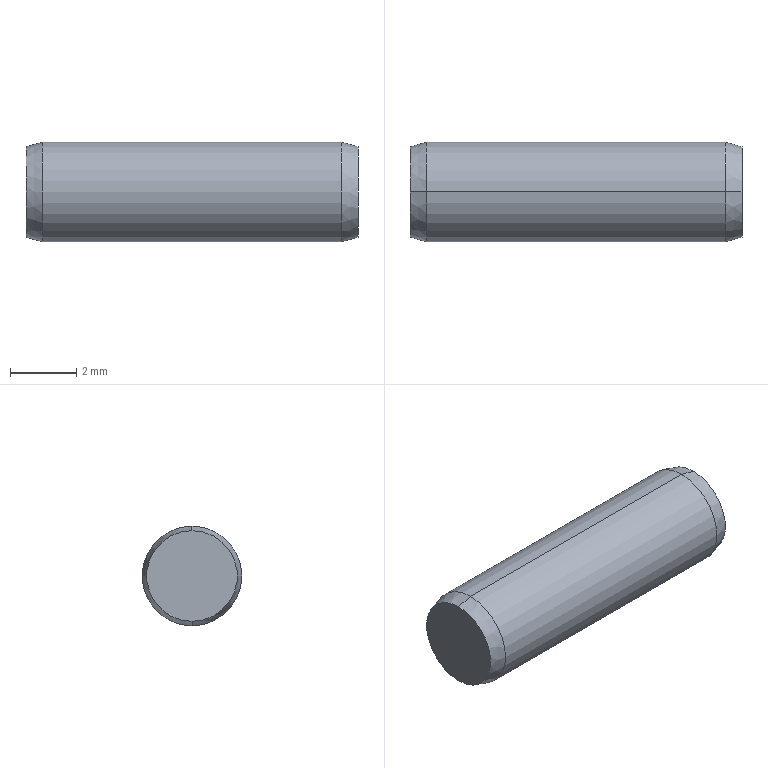Part | NX | features BREP 1 | 1 solid | 8 faces | box 10 x 3 x 3 mm | volume 70.073 mm3 | cone 4 | cylinder 2 | plane 2 | commonest cylinder face diameters 3 x2
STEP:
#1=CARTESIAN_POINT('',(-1.,0.,-1.5));
#2=VERTEX_POINT('',#1);
#3=CARTESIAN_POINT('',(8.,0.,-1.5));
#4=VERTEX_POINT('',#3);
#5=CARTESIAN_POINT('',(0.,0.,-1.5));
#6=DIRECTION('',(-1.,0.,0.));
#7=VECTOR('',#6,1000.);
#8=LINE('',#5,#7);
#9=EDGE_CURVE('',#2,#4,#8,.F.);
#10=ORIENTED_EDGE('',*,*,#9,.T.);
#11=CARTESIAN_POINT('',(8.,0.,1.5));
#12=VERTEX_POINT('',#11);
#13=CARTESIAN_POINT('',(8.,0.,0.));
#14=DIRECTION('',(-1.,0.,0.));
#15=DIRECTION('',(0.,0.,1.));
#16=AXIS2_PLACEMENT_3D('',#13,#14,#15);
#17=CIRCLE('',#16,1.5);
#18=EDGE_CURVE('',#4,#12,#17,.T.);
#19=ORIENTED_EDGE('',*,*,#18,.T.);
#20=CARTESIAN_POINT('',(-1.,0.,1.5));
#21=VERTEX_POINT('',#20);
#22=CARTESIAN_POINT('',(0.,0.,1.5));
#23=DIRECTION('',(-1.,0.,0.));
#24=VECTOR('',#23,1000.);
#25=LINE('',#22,#24);
#26=EDGE_CURVE('',#21,#12,#25,.F.);
#27=ORIENTED_EDGE('',*,*,#26,.F.);
#28=CARTESIAN_POINT('',(-1.,0.,0.));
#29=DIRECTION('',(-1.,0.,0.));
#30=DIRECTION('',(0.,0.,1.));
#31=AXIS2_PLACEMENT_3D('',#28,#29,#30);
#32=CIRCLE('',#31,1.5);
#33=EDGE_CURVE('',#2,#21,#32,.T.);
#34=ORIENTED_EDGE('',*,*,#33,.F.);
#35=EDGE_LOOP('',(#10,#19,#27,#34));
#36=FACE_BOUND('',#35,.T.);
#37=CARTESIAN_POINT('',(0.,0.,0.));
#38=DIRECTION('',(-1.,0.,0.));
#39=DIRECTION('',(0.,0.,1.));
#40=AXIS2_PLACEMENT_3D('',#37,#38,#39);
#41=CYLINDRICAL_SURFACE('',#40,1.5);
#42=ADVANCED_FACE('',(#36),#41,.T.);
#43=CARTESIAN_POINT('',(-1.5,0.,1.366));
#44=VERTEX_POINT('',#43);
#45=CARTESIAN_POINT('',(-1.,0.,1.5));
#46=DIRECTION('',(0.9659,0.,0.2588));
#47=VECTOR('',#46,1000.);
#48=LINE('',#45,#47);
#49=EDGE_CURVE('',#44,#21,#48,.T.);
#50=ORIENTED_EDGE('',*,*,#49,.F.);
#51=CARTESIAN_POINT('',(-1.5,0.,-1.366));
#52=VERTEX_POINT('',#51);
#53=CARTESIAN_POINT('',(-1.5,0.,0.));
#54=DIRECTION('',(-1.,0.,0.));
#55=DIRECTION('',(0.,0.,1.));
#56=AXIS2_PLACEMENT_3D('',#53,#54,#55);
#57=CIRCLE('',#56,1.366);
#58=EDGE_CURVE('',#52,#44,#57,.T.);
#59=ORIENTED_EDGE('',*,*,#58,.F.);
#60=CARTESIAN_POINT('',(-1.,0.,-1.5));
#61=DIRECTION('',(0.9659,0.,-0.2588));
#62=VECTOR('',#61,1000.);
#63=LINE('',#60,#62);
#64=EDGE_CURVE('',#52,#2,#63,.T.);
#65=ORIENTED_EDGE('',*,*,#64,.T.);
#66=ORIENTED_EDGE('',*,*,#33,.T.);
#67=EDGE_LOOP('',(#50,#59,#65,#66));
#68=FACE_BOUND('',#67,.T.);
#69=CARTESIAN_POINT('',(-1.,0.,0.));
#70=DIRECTION('',(1.,0.,0.));
#71=DIRECTION('',(0.,0.,-1.));
#72=AXIS2_PLACEMENT_3D('',#69,#70,#71);
#73=CONICAL_SURFACE('',#72,1.5,0.2618);
#74=ADVANCED_FACE('',(#68),#73,.T.);
#75=ORIENTED_EDGE('',*,*,#58,.T.);
#76=CARTESIAN_POINT('',(-1.5,0.,0.));
#77=DIRECTION('',(-1.,0.,0.));
#78=DIRECTION('',(0.,0.,1.));
#79=AXIS2_PLACEMENT_3D('',#76,#77,#78);
#80=CIRCLE('',#79,1.366);
#81=EDGE_CURVE('',#44,#52,#80,.T.);
#82=ORIENTED_EDGE('',*,*,#81,.T.);
#83=EDGE_LOOP('',(#75,#82));
#84=FACE_BOUND('',#83,.T.);
#85=CARTESIAN_POINT('',(-1.5,1.366,0.));
#86=DIRECTION('',(1.,0.,0.));
#87=DIRECTION('',(0.,0.,-1.));
#88=AXIS2_PLACEMENT_3D('',#85,#86,#87);
#89=PLANE('',#88);
#90=ADVANCED_FACE('',(#84),#89,.F.);
#91=CARTESIAN_POINT('',(8.5,0.,1.366));
#92=VERTEX_POINT('',#91);
#93=CARTESIAN_POINT('',(8.5,0.,-1.366));
#94=VERTEX_POINT('',#93);
#95=CARTESIAN_POINT('',(8.5,0.,0.));
#96=DIRECTION('',(-1.,0.,0.));
#97=DIRECTION('',(0.,0.,1.));
#98=AXIS2_PLACEMENT_3D('',#95,#96,#97);
#99=CIRCLE('',#98,1.366);
#100=EDGE_CURVE('',#92,#94,#99,.T.);
#101=ORIENTED_EDGE('',*,*,#100,.F.);
#102=CARTESIAN_POINT('',(8.5,0.,0.));
#103=DIRECTION('',(-1.,0.,0.));
#104=DIRECTION('',(0.,0.,1.));
#105=AXIS2_PLACEMENT_3D('',#102,#103,#104);
#106=CIRCLE('',#105,1.366);
#107=EDGE_CURVE('',#94,#92,#106,.T.);
#108=ORIENTED_EDGE('',*,*,#107,.F.);
#109=EDGE_LOOP('',(#101,#108));
#110=FACE_BOUND('',#109,.T.);
#111=CARTESIAN_POINT('',(8.5,1.366,0.));
#112=DIRECTION('',(-1.,0.,0.));
#113=DIRECTION('',(0.,0.,1.));
#114=AXIS2_PLACEMENT_3D('',#111,#112,#113);
#115=PLANE('',#114);
#116=ADVANCED_FACE('',(#110),#115,.F.);
#117=CARTESIAN_POINT('',(8.5,0.,-1.366));
#118=DIRECTION('',(-0.9659,0.,-0.2588));
#119=VECTOR('',#118,1000.);
#120=LINE('',#117,#119);
#121=EDGE_CURVE('',#4,#94,#120,.F.);
#122=ORIENTED_EDGE('',*,*,#121,.T.);
#123=ORIENTED_EDGE('',*,*,#107,.T.);
#124=CARTESIAN_POINT('',(8.5,0.,1.366));
#125=DIRECTION('',(-0.9659,0.,0.2588));
#126=VECTOR('',#125,1000.);
#127=LINE('',#124,#126);
#128=EDGE_CURVE('',#12,#92,#127,.F.);
#129=ORIENTED_EDGE('',*,*,#128,.F.);
#130=ORIENTED_EDGE('',*,*,#18,.F.);
#131=EDGE_LOOP('',(#122,#123,#129,#130));
#132=FACE_BOUND('',#131,.T.);
#133=CARTESIAN_POINT('',(8.5,0.,0.));
#134=DIRECTION('',(-1.,0.,0.));
#135=DIRECTION('',(0.,0.,1.));
#136=AXIS2_PLACEMENT_3D('',#133,#134,#135);
#137=CONICAL_SURFACE('',#136,1.366,0.2618);
#138=ADVANCED_FACE('',(#132),#137,.T.);
#139=ORIENTED_EDGE('',*,*,#100,.T.);
#140=ORIENTED_EDGE('',*,*,#121,.F.);
#141=CARTESIAN_POINT('',(8.,0.,0.));
#142=DIRECTION('',(-1.,0.,0.));
#143=DIRECTION('',(0.,0.,1.));
#144=AXIS2_PLACEMENT_3D('',#141,#142,#143);
#145=CIRCLE('',#144,1.5);
#146=EDGE_CURVE('',#12,#4,#145,.T.);
#147=ORIENTED_EDGE('',*,*,#146,.F.);
#148=ORIENTED_EDGE('',*,*,#128,.T.);
#149=EDGE_LOOP('',(#139,#140,#147,#148));
#150=FACE_BOUND('',#149,.T.);
#151=CARTESIAN_POINT('',(8.5,0.,0.));
#152=DIRECTION('',(-1.,0.,0.));
#153=DIRECTION('',(0.,0.,1.));
#154=AXIS2_PLACEMENT_3D('',#151,#152,#153);
#155=CONICAL_SURFACE('',#154,1.366,0.2618);
#156=ADVANCED_FACE('',(#150),#155,.T.);
#157=ORIENTED_EDGE('',*,*,#81,.F.);
#158=ORIENTED_EDGE('',*,*,#49,.T.);
#159=CARTESIAN_POINT('',(-1.,0.,0.));
#160=DIRECTION('',(-1.,0.,0.));
#161=DIRECTION('',(0.,0.,1.));
#162=AXIS2_PLACEMENT_3D('',#159,#160,#161);
#163=CIRCLE('',#162,1.5);
#164=EDGE_CURVE('',#21,#2,#163,.T.);
#165=ORIENTED_EDGE('',*,*,#164,.T.);
#166=ORIENTED_EDGE('',*,*,#64,.F.);
#167=EDGE_LOOP('',(#157,#158,#165,#166));
#168=FACE_BOUND('',#167,.T.);
#169=CARTESIAN_POINT('',(-1.,0.,0.));
#170=DIRECTION('',(1.,0.,0.));
#171=DIRECTION('',(0.,0.,-1.));
#172=AXIS2_PLACEMENT_3D('',#169,#170,#171);
#173=CONICAL_SURFACE('',#172,1.5,0.2618);
#174=ADVANCED_FACE('',(#168),#173,.T.);
#175=ORIENTED_EDGE('',*,*,#146,.T.);
#176=ORIENTED_EDGE('',*,*,#9,.F.);
#177=ORIENTED_EDGE('',*,*,#164,.F.);
#178=ORIENTED_EDGE('',*,*,#26,.T.);
#179=EDGE_LOOP('',(#175,#176,#177,#178));
#180=FACE_BOUND('',#179,.T.);
#181=CARTESIAN_POINT('',(0.,0.,0.));
#182=DIRECTION('',(-1.,0.,0.));
#183=DIRECTION('',(0.,0.,1.));
#184=AXIS2_PLACEMENT_3D('',#181,#182,#183);
#185=CYLINDRICAL_SURFACE('',#184,1.5);
#186=ADVANCED_FACE('',(#180),#185,.T.);
#187=CLOSED_SHELL('',(#42,#74,#90,#116,#138,#156,#174,#186));
#188=MANIFOLD_SOLID_BREP('',#187);
#189=(LENGTH_UNIT()NAMED_UNIT(*)SI_UNIT(.MILLI.,.METRE.));
#190=UNCERTAINTY_MEASURE_WITH_UNIT(LENGTH_MEASURE(0.00001),#189,'','');
#191=(NAMED_UNIT(*)PLANE_ANGLE_UNIT()SI_UNIT($,.RADIAN.));
#192=(NAMED_UNIT(*)SI_UNIT($,.STERADIAN.)SOLID_ANGLE_UNIT());
#193=(GEOMETRIC_REPRESENTATION_CONTEXT(3)GLOBAL_UNCERTAINTY_ASSIGNED_CONTEXT((#190))GLOBAL_UNIT_ASSIGNED_CONTEXT((#189,#191,#192))REPRESENTATION_CONTEXT('',''));
#194=ADVANCED_BREP_SHAPE_REPRESENTATION('',(#188),#193);